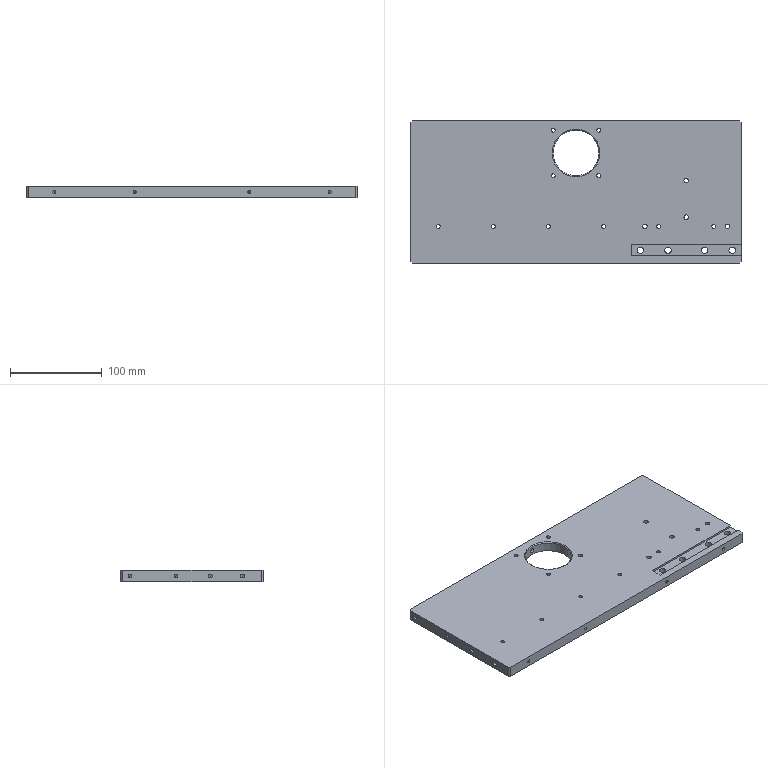Part | 1 solid | 68 faces | box 360 x 155 x 12 mm | volume 635278 mm3 | cylinder 34 | cone 20 | plane 14 | commonest cylinder face diameters 4.2 x18 5 x7 3.3 x4 7 x4 50 x1